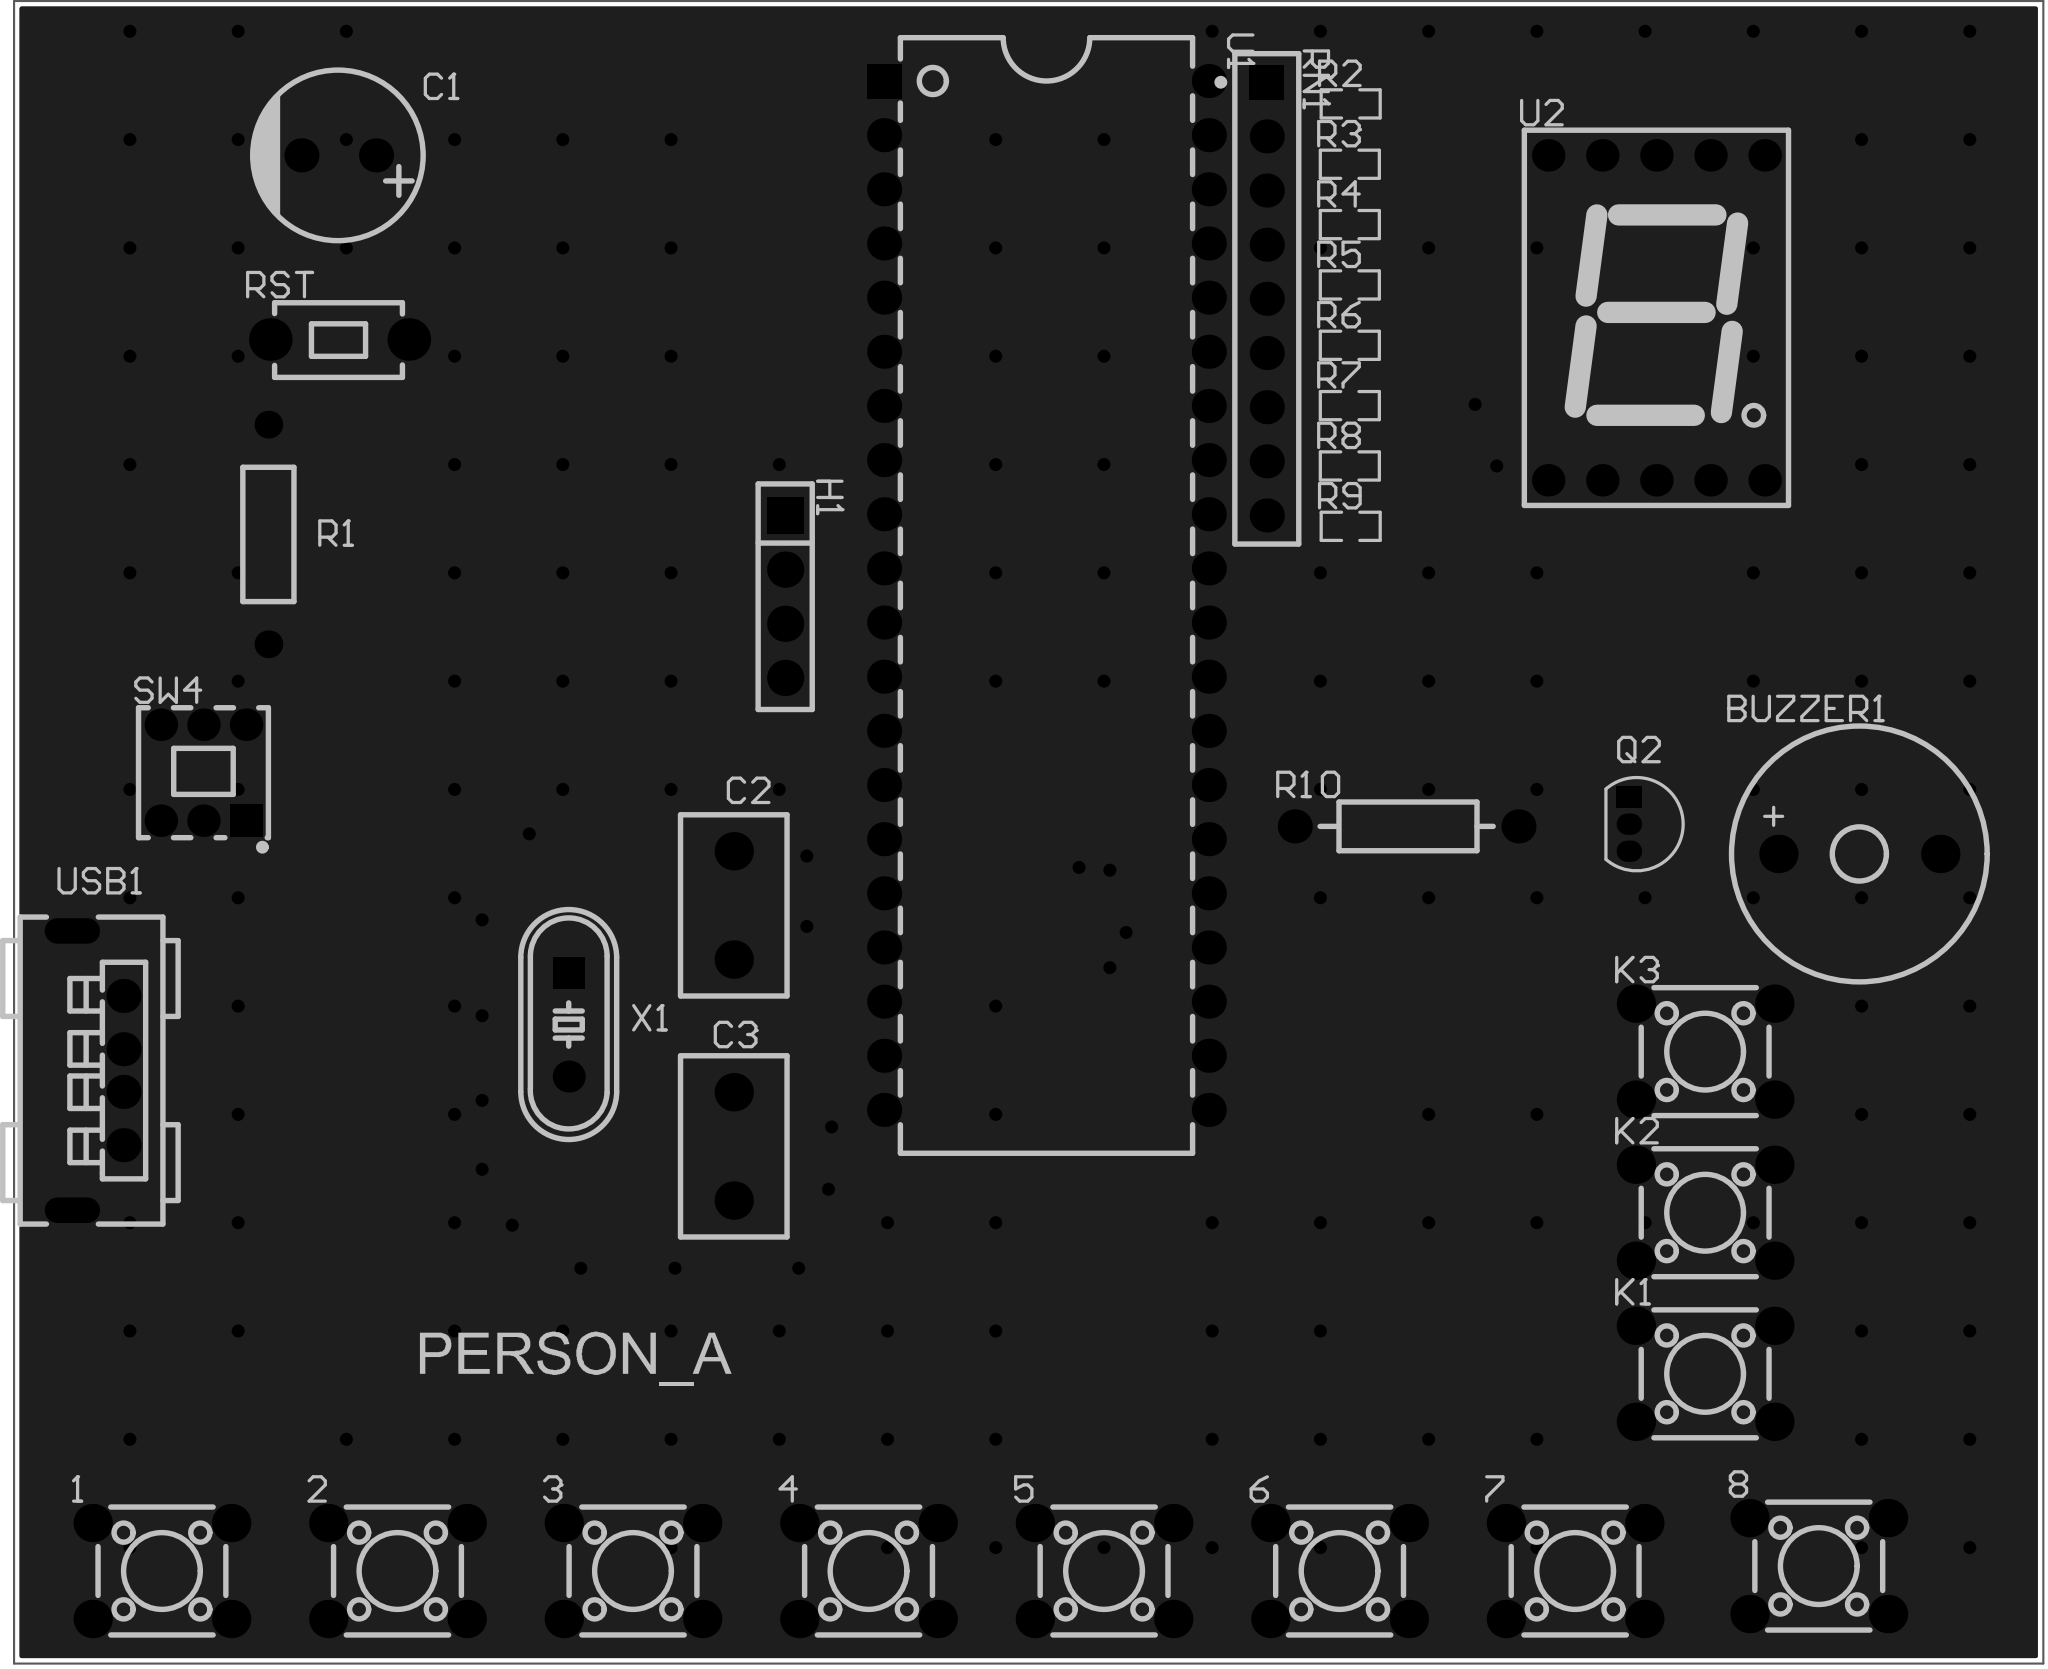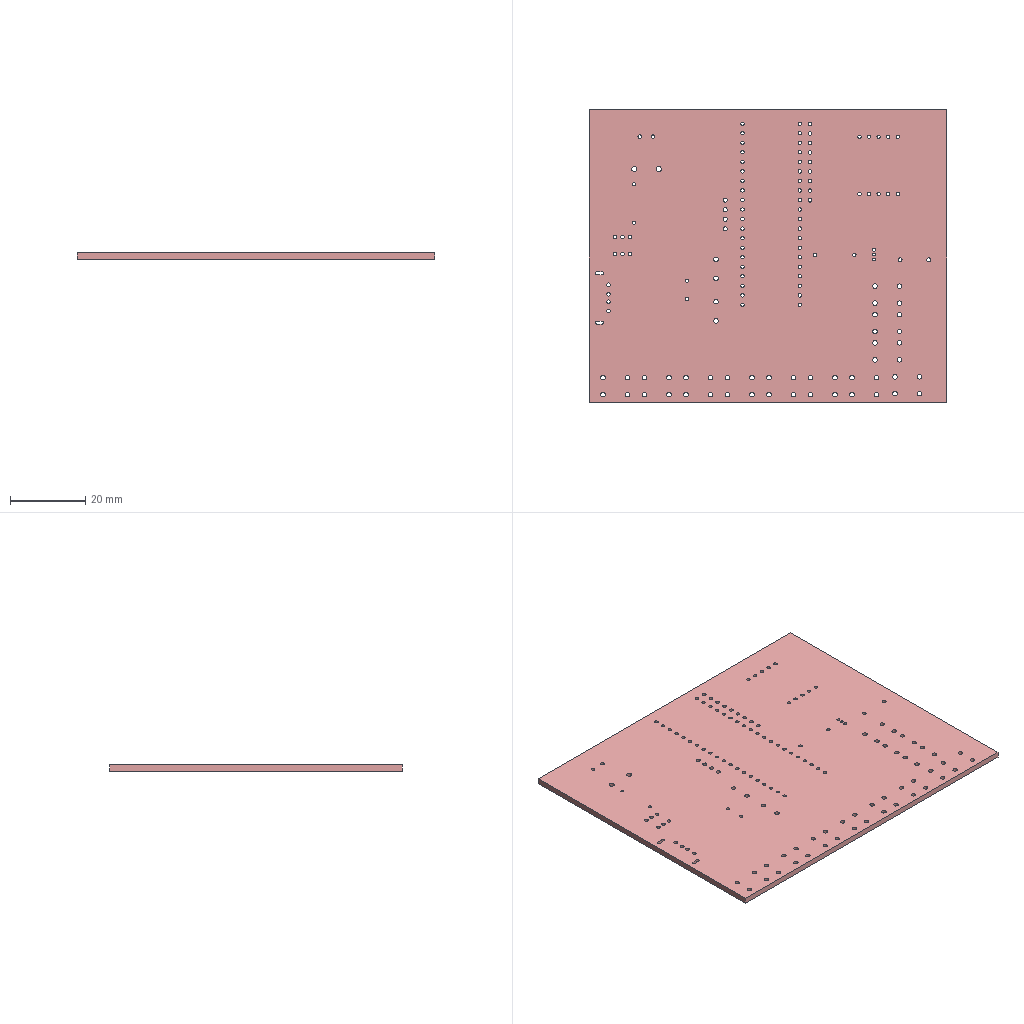Circuit board layout | Altium Designer | box 95.2 x 78 x 1.6 mm
Layer stack:
# Altium Designer layer stack of  (unit mm; dielectric type: 0 none, 1 core, 2 prepreg, 3 surface material)
index,name,kind,layer,copper_thickness_mm,dielectric_type,dielectric_thickness_mm,dielectric_material,dielectric_constant
0,Top Paste Mask Layer,other,,,,,,
1,Top Silkscreen Layer,other,,,,,,
2,Top Solder Mask Layer,dielectric,,,3,0.01,,3.3
3,Top Layer,copper,Top Layer,0.035,,,,
4,Dielectric1,dielectric,,,3,1.51,FR4,4.5
5,Bottom Layer,copper,Bottom Layer,0.035,,,,
6,Bottom Solder Mask Layer,dielectric,,,3,0.01,,3.3
7,Bottom Silkscreen Layer,other,,,,,,
8,Bottom Paste Mask Layer,other,,,,,,
# drill layer pairs: low layer,high layer
drill_pair,Top Layer,Bottom Layer
Part placement:
Designator,Comment,Layer,Footprint,Center-X(mm),Center-Y(mm),Rotation
BUZZER1,2.4kHz,TopLayer,BUZ-TH_BD12.0-P7.60-D0.6-FD,181.483,122.682,0
C1,10uF,TopLayer,CAP-TH_BD8.0-P3.50-D0.6-FD,110.109,155.448,180
C2,30pF,TopLayer,CAP-TH_L8.5-W5.0-P5.00-D1.2,128.651,120.269,270
C3,30pF,TopLayer,CAP-TH_L8.5-W5.0-P5.00-D1.2,128.651,108.966,90
Q2,S8550,TopLayer,TO-92-3_L4.5-W3.5-P1.27-L,170.688,124.079,270
R1,10kΩ,TopLayer,RES-TH_BD2.4-L6.3-P10.30-D0.6,106.807,137.668,90
R2,470,TopLayer,R0603,157.607,157.861,0
R3,470,TopLayer,R0603,157.567,155.031,0
R4,470,TopLayer,R0603,157.567,152.2,0
R5,470,TopLayer,R0603,157.567,149.37,0
R6,470,TopLayer,R0603,157.567,146.54,0
R7,470,TopLayer,R0603,157.567,143.71,0
R8,470,TopLayer,R0603,157.567,140.879,0
R9,470,TopLayer,R0603,157.607,138.049,0
R10,4.7K,TopLayer,RES-TH_BD2.2-L6.5-P10.50-D0.6,160.234,123.975,0
SW4,5.8 ZSGT,TopLayer,SW-TH_5.8ZSGT,103.759,126.492,0
U1,STC89C52RC-40I-PDIP40,TopLayer,DIP-40_L52.0-W13.7-P2.54-LS15.2-BL,143.329,134.805,270
U2,TDSR1360,TopLayer,LED-SEG-TH_10P-L17.6-W12.4-P2.54-S15.24-BL,171.958,147.828,0
X1,12MHz,TopLayer,HC-49US_L11.5-W4.5-P4.88,120.904,114.681,270
RST,,TopLayer,Key_TH_3.5x6x4.3,110.147,146.812,0
1,TS665CJ,TopLayer,SW-TH_4P-L6.0-W6.0-P4.50-LS6.5,101.81,89.05,0
2,TS665CJ,TopLayer,SW-TH_4P-L6.0-W6.0-P4.50-LS6.5,112.866,89.05,0
3,TS665CJ,TopLayer,SW-TH_4P-L6.0-W6.0-P4.50-LS6.5,123.921,89.05,0
4,TS665CJ,TopLayer,SW-TH_4P-L6.0-W6.0-P4.50-LS6.5,134.976,89.05,0
5,TS665CJ,TopLayer,SW-TH_4P-L6.0-W6.0-P4.50-LS6.5,146.031,89.05,0
6,TS665CJ,TopLayer,SW-TH_4P-L6.0-W6.0-P4.50-LS6.5,157.087,89.05,0
7,TS665CJ,TopLayer,SW-TH_4P-L6.0-W6.0-P4.50-LS6.5,168.142,89.05,0
8,TS665CJ,TopLayer,SW-TH_4P-L6.0-W6.0-P4.50-LS6.5,179.578,89.281,0
K1,TS665CJ,TopLayer,SW-TH_4P-L6.0-W6.0-P4.50-LS6.5,174.244,98.298,0
K2,TS665CJ,TopLayer,SW-TH_4P-L6.0-W6.0-P4.50-LS6.5,174.244,105.855,0
K3,TS665CJ,TopLayer,SW-TH_4P-L6.0-W6.0-P4.50-LS6.5,174.244,113.411,0
USB1,AF 180°ZJB13.7,TopLayer,USB-A-TH_AF-ZJB13.7,98.806,112.522,270
H1,,TopLayer,HDR-TH_4P-P2.54-V-F,131.064,134.747,270
RN1,-,TopLayer,RES-ARRAY-TH_9P-P2.54-D1.0,153.67,148.717,270
Pad and via stacks:
# Altium Designer via and pad stacks of  (unit mm). Each distinct definition once, with the count of objects using it.
# via: kind,start_layer,end_layer,hole_mm,diameter_mm,mode(0 simple;1 top-mid-bottom;2 full stack),diameter_per_layer,count,example_net
# pad: kind,layer,hole_mm,hole_type(0 round;1 square;2 slot),plating,top_size,top_shape(1 round;2 rect;3 octagon;9 rounded rect),mid_size,bottom_size,mode,footprint,size_per_layer,count,example
pad,Multi-Layer,1,0,plated,1.8x1.8,1,1.8x1.8,1.8x1.8,0,BUZ-TH_BD12.0-P7.60-D0.6-FD,,2,BUZZER1.2
pad,Multi-Layer,1,0,plated,1.6x1.6,1,1.6x1.6,1.6x1.6,0,CAP-TH_BD8.0-P3.50-D0.6-FD,,2,C1.2
pad,Multi-Layer,1.2,0,plated,1.8x1.8,1,1.8x1.8,1.8x1.8,0,CAP-TH_L8.5-W5.0-P5.00-D1.2,,4,C2.1
pad,Multi-Layer,0.7,2,plated,1x1.2,2,1x1.2,1x1.2,0,TO-92-3_L4.5-W3.5-P1.27-L,,1,Q2.1
pad,Multi-Layer,0.7,2,plated,1x1.2,1,1x1.2,1x1.2,0,TO-92-3_L4.5-W3.5-P1.27-L,,2,Q2.2
pad,Multi-Layer,0.8,0,plated,1.3x1.3,1,1.3x1.3,1.3x1.3,0,RES-TH_BD2.4-L6.3-P10.30-D0.6,,2,R1.1
pad,Multi-Layer,0.9144,0,plated,1.6x1.6,1,1.6x1.6,1.6x1.6,0,RES-TH_BD2.2-L6.5-P10.50-D0.6,,2,R10.1
pad,Multi-Layer,1,0,plated,1.524x1.524,1,1.524x1.524,1.524x1.524,0,SW-TH_5.8ZSGT,,5,SW4.4
pad,Multi-Layer,1,0,plated,1.524x1.524,2,1.524x1.524,1.524x1.524,0,SW-TH_5.8ZSGT,,1,SW4.1
pad,Multi-Layer,0.889,0,plated,1.6x1.6,1,1.6x1.6,1.6x1.6,0,DIP-40_L52.0-W13.7-P2.54-LS15.2-BL,,39,U1.31
pad,Multi-Layer,0.889,0,plated,1.6x1.6,2,1.6x1.6,1.6x1.6,0,DIP-40_L52.0-W13.7-P2.54-LS15.2-BL,,1,U1.1
pad,Multi-Layer,0.9144,0,plated,1.524x1.524,1,1.524x1.524,1.524x1.524,0,LED-SEG-TH_10P-L17.6-W12.4-P2.54-S15.24-BL,,10,U2.10
pad,Multi-Layer,0.9,0,plated,1.5x1.5,2,1.5x1.5,1.5x1.5,0,HC-49US_L11.5-W4.5-P4.88,,1,X1.1
pad,Multi-Layer,0.9,0,plated,1.5x1.5,1,1.5x1.5,1.5x1.5,0,HC-49US_L11.5-W4.5-P4.88,,1,X1.2
pad,Multi-Layer,1.399,0,plated,1.999x1.999,1,1.999x1.999,1.999x1.999,0,Key_TH_3.5x6x4.3,,2,RST.A
pad,Multi-Layer,1.2,0,plated,1.8x1.8,1,1.8x1.8,1.8x1.8,0,SW-TH_4P-L6.0-W6.0-P4.50-LS6.5,,44,1.1
pad,Multi-Layer,1,0,plated,1.6x1.6,1,1.6x1.6,1.6x1.6,0,USB-A-TH_AF-ZJB13.7,,4,USB1.1
pad,Multi-Layer,0.8,2,plated,1.2x2.6,1,1.2x2.6,1.2x2.6,0,USB-A-TH_AF-ZJB13.7,,2,USB1.5
pad,Multi-Layer,1.1,0,plated,1.7x1.7,2,1.7x1.7,1.7x1.7,0,HDR-TH_4P-P2.54-V-F,,1,H1.1
pad,Multi-Layer,1.1,0,plated,1.7x1.7,1,1.7x1.7,1.7x1.7,0,HDR-TH_4P-P2.54-V-F,,3,H1.2
pad,Multi-Layer,1,0,plated,1.6x1.6,2,1.6x1.6,1.6x1.6,0,RES-ARRAY-TH_9P-P2.54-D1.0,,1,RN1.1
pad,Multi-Layer,1,0,plated,1.6x1.6,1,1.6x1.6,1.6x1.6,0,RES-ARRAY-TH_9P-P2.54-D1.0,,8,RN1.2
pad,Top Layer,0,0,plated,0.8065x0.864,2,0.8065x0.864,0.8065x0.864,0,R0603,,16,R2.2
via,Top Layer,Bottom Layer,0.3048,0.61,0,,181,G
Copper pours:
name,layer,net,type(0 solid;1 hatched;2 none)
Bottom Layer-GND,Bottom Layer,GND,0
Top Layer-GND,Top Layer,GND,0